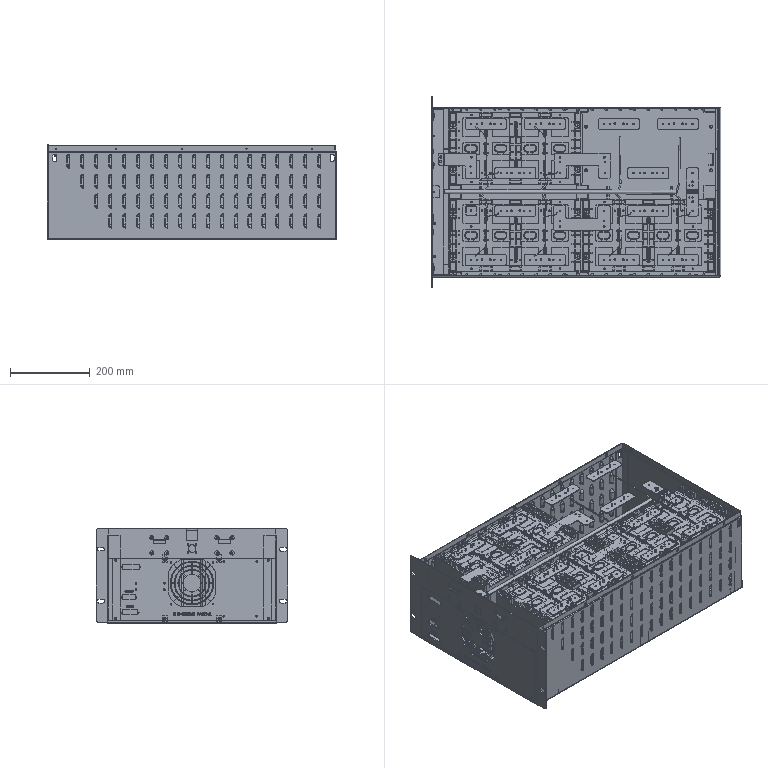Part | NX | features BREP 69 | 80 solids | 10882 faces | volume 33839951 mm3 | plane 5886 | cylinder 3390 | sphere 564 | torus 366 | spline 356 | cone 320 | commonest cylinder face diameters 4 x769 6 x546 10 x276 3 x229 12 x158 2 x156